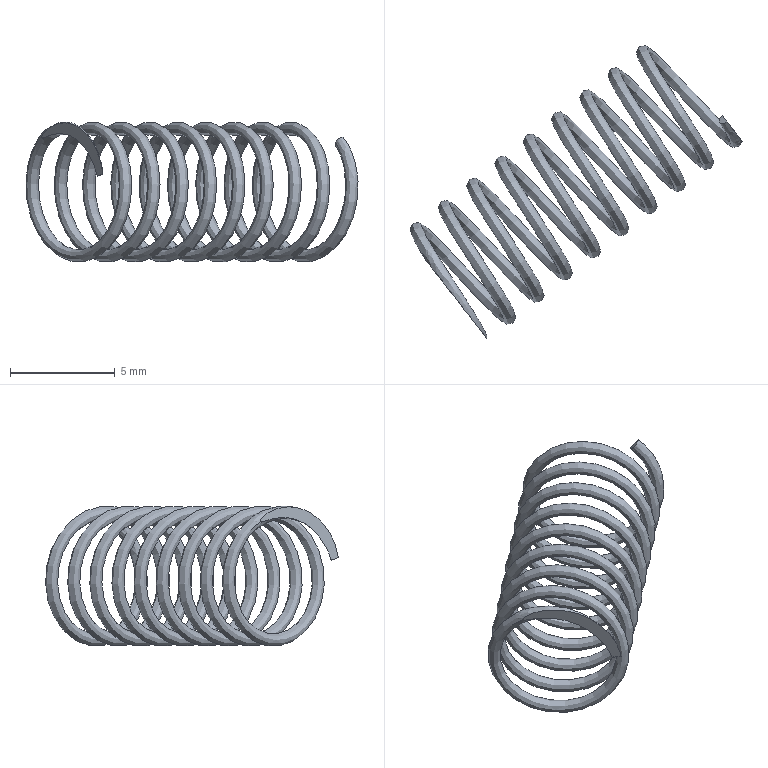Part | NX | features BREP 1 | 1 solid | 5 faces | volume 48.548 mm3 | plane 4 | spline 1
STEP:
#1=CARTESIAN_POINT('',(-3.477,87.158,-116.985));
#2=VERTEX_POINT('',#1);
#3=CARTESIAN_POINT('',(-3.213,86.82,-116.865));
#4=VERTEX_POINT('',#3);
#5=CARTESIAN_POINT('',(-3.345,86.989,-116.925));
#6=DIRECTION('',(0.5927,-0.7586,0.2704));
#7=VECTOR('',#6,1000.);
#8=LINE('',#5,#7);
#9=EDGE_CURVE('',#2,#4,#8,.T.);
#10=ORIENTED_EDGE('',*,*,#9,.F.);
#11=CARTESIAN_POINT('',(-3.213,86.82,-116.865));
#12=CARTESIAN_POINT('',(-3.181,86.983,-116.896));
#13=CARTESIAN_POINT('',(-3.311,87.149,-116.955));
#14=CARTESIAN_POINT('',(-3.477,87.157,-116.985));
#15=B_SPLINE_CURVE_WITH_KNOTS('',3,(#11,#12,#13,#14),.UNSPECIFIED.,.F.,.F.,(4,4),(0.,0.0004991),.UNSPECIFIED.);
#16=EDGE_CURVE('',#4,#2,#15,.T.);
#17=ORIENTED_EDGE('',*,*,#16,.F.);
#18=EDGE_LOOP('',(#10,#17));
#19=FACE_BOUND('',#18,.T.);
#20=CARTESIAN_POINT('',(-3.502,86.866,-116.925));
#21=DIRECTION('',(-0.1665,0.2131,0.9627));
#22=DIRECTION('',(0.788,0.6157,0.));
#23=AXIS2_PLACEMENT_3D('',#20,#21,#22);
#24=PLANE('',#23);
#25=ADVANCED_FACE('',(#19),#24,.F.);
#26=CARTESIAN_POINT('',(8.032,97.44,-115.592));
#27=VERTEX_POINT('',#26);
#28=CARTESIAN_POINT('',(7.91,97.109,-115.357));
#29=VERTEX_POINT('',#28);
#30=CARTESIAN_POINT('',(8.147,97.294,-115.357));
#31=DIRECTION('',(-0.4831,0.6183,0.6199));
#32=DIRECTION('',(-0.788,-0.6157,0.));
#33=AXIS2_PLACEMENT_3D('',#30,#31,#32);
#34=CIRCLE('',#33,0.3);
#35=EDGE_CURVE('',#27,#29,#34,.T.);
#36=ORIENTED_EDGE('',*,*,#35,.F.);
#37=CARTESIAN_POINT('',(8.261,97.147,-115.121));
#38=VERTEX_POINT('',#37);
#39=CARTESIAN_POINT('',(8.032,97.44,-115.592));
#40=CARTESIAN_POINT('',(8.311,97.083,-115.95));
#41=CARTESIAN_POINT('',(8.572,96.75,-116.555));
#42=CARTESIAN_POINT('',(8.721,96.559,-117.384));
#43=CARTESIAN_POINT('',(8.758,96.511,-117.734));
#44=CARTESIAN_POINT('',(8.776,96.489,-118.029));
#45=CARTESIAN_POINT('',(8.787,96.475,-118.188));
#46=CARTESIAN_POINT('',(8.798,96.46,-118.373));
#47=CARTESIAN_POINT('',(8.887,96.346,-118.311));
#48=CARTESIAN_POINT('',(8.925,96.298,-118.048));
#49=CARTESIAN_POINT('',(8.977,96.232,-117.718));
#50=CARTESIAN_POINT('',(8.979,96.228,-117.148));
#51=CARTESIAN_POINT('',(8.889,96.344,-116.453));
#52=CARTESIAN_POINT('',(8.641,96.662,-115.706));
#53=CARTESIAN_POINT('',(8.398,96.972,-115.297));
#54=CARTESIAN_POINT('',(8.261,97.147,-115.121));
#55=B_SPLINE_CURVE_WITH_KNOTS('',3,(#39,#40,#41,#42,#43,#44,#45,#46,#47,#48,#49,#50,#51,#52,#53,#54),.UNSPECIFIED.,.F.,.F.,(4,1,1,1,1,1,1,1,1,1,1,1,1,4),(0.,0.001724,0.002155,0.002586,0.002802,0.003017,0.003125,0.003233,0.003448,0.003879,0.00431,0.005172,0.006034,0.006896),.UNSPECIFIED.);
#56=EDGE_CURVE('',#27,#38,#55,.T.);
#57=ORIENTED_EDGE('',*,*,#56,.T.);
#58=CARTESIAN_POINT('',(8.147,97.294,-115.357));
#59=DIRECTION('',(-0.4831,0.6183,0.6199));
#60=DIRECTION('',(-0.788,-0.6157,0.));
#61=AXIS2_PLACEMENT_3D('',#58,#59,#60);
#62=CIRCLE('',#61,0.3);
#63=EDGE_CURVE('',#29,#38,#62,.T.);
#64=ORIENTED_EDGE('',*,*,#63,.F.);
#65=EDGE_LOOP('',(#36,#57,#64));
#66=FACE_BOUND('',#65,.T.);
#67=CARTESIAN_POINT('',(-3.213,86.82,-116.865));
#68=CARTESIAN_POINT('',(-3.27,86.893,-116.4));
#69=CARTESIAN_POINT('',(-3.527,87.222,-115.533));
#70=CARTESIAN_POINT('',(-4.113,87.971,-114.786));
#71=CARTESIAN_POINT('',(-4.66,88.672,-114.483));
#72=CARTESIAN_POINT('',(-5.095,89.229,-114.412));
#73=CARTESIAN_POINT('',(-5.529,89.784,-114.512));
#74=CARTESIAN_POINT('',(-5.831,90.171,-114.709));
#75=CARTESIAN_POINT('',(-6.016,90.408,-114.909));
#76=CARTESIAN_POINT('',(-6.078,90.487,-115.));
#77=CARTESIAN_POINT('',(-6.139,90.566,-115.105));
#78=CARTESIAN_POINT('',(-6.087,90.498,-115.194));
#79=CARTESIAN_POINT('',(-5.948,90.32,-115.1));
#80=CARTESIAN_POINT('',(-5.779,90.104,-115.048));
#81=CARTESIAN_POINT('',(-5.487,89.73,-114.95));
#82=CARTESIAN_POINT('',(-5.125,89.268,-114.935));
#83=CARTESIAN_POINT('',(-4.254,88.152,-115.192));
#84=CARTESIAN_POINT('',(-3.686,87.426,-116.093));
#85=CARTESIAN_POINT('',(-3.477,87.158,-116.985));
#86=B_SPLINE_CURVE_WITH_KNOTS('',3,(#67,#68,#69,#70,#71,#72,#73,#74,#75,#76,#77,#78,#79,#80,#81,#82,#83,#84,#85),.UNSPECIFIED.,.F.,.F.,(4,1,1,1,1,1,1,1,1,1,1,1,1,1,1,1,4),(0.,0.001414,0.002829,0.003536,0.004243,0.00495,0.005658,0.005834,0.006011,0.0061,0.006188,0.006365,0.006719,0.007072,0.007779,0.008487,0.01132),.UNSPECIFIED.);
#87=EDGE_CURVE('',#4,#2,#86,.T.);
#88=ORIENTED_EDGE('',*,*,#87,.F.);
#89=ORIENTED_EDGE('',*,*,#16,.T.);
#90=EDGE_LOOP('',(#88,#89));
#91=FACE_BOUND('',#90,.T.);
#92=CARTESIAN_POINT('',(7.91,97.109,-115.357));
#93=CARTESIAN_POINT('',(8.648,95.932,-116.448));
#94=CARTESIAN_POINT('',(8.379,96.045,-118.191));
#95=CARTESIAN_POINT('',(8.11,96.158,-119.933));
#96=CARTESIAN_POINT('',(6.99,97.359,-120.584));
#97=CARTESIAN_POINT('',(5.87,98.56,-121.235));
#98=CARTESIAN_POINT('',(4.907,99.561,-120.143));
#99=CARTESIAN_POINT('',(3.944,100.562,-119.052));
#100=CARTESIAN_POINT('',(3.988,100.274,-117.309));
#101=CARTESIAN_POINT('',(4.032,99.985,-115.567));
#102=CARTESIAN_POINT('',(4.927,98.608,-114.916));
#103=CARTESIAN_POINT('',(5.821,97.231,-114.265));
#104=CARTESIAN_POINT('',(6.559,96.054,-115.357));
#105=CARTESIAN_POINT('',(7.298,94.877,-116.448));
#106=CARTESIAN_POINT('',(7.028,94.99,-118.191));
#107=CARTESIAN_POINT('',(6.759,95.102,-119.933));
#108=CARTESIAN_POINT('',(5.639,96.304,-120.584));
#109=CARTESIAN_POINT('',(4.519,97.505,-121.235));
#110=CARTESIAN_POINT('',(3.556,98.506,-120.143));
#111=CARTESIAN_POINT('',(2.593,99.507,-119.052));
#112=CARTESIAN_POINT('',(2.637,99.218,-117.309));
#113=CARTESIAN_POINT('',(2.681,98.93,-115.567));
#114=CARTESIAN_POINT('',(3.576,97.552,-114.916));
#115=CARTESIAN_POINT('',(4.47,96.175,-114.265));
#116=CARTESIAN_POINT('',(5.209,94.998,-115.357));
#117=CARTESIAN_POINT('',(5.947,93.822,-116.448));
#118=CARTESIAN_POINT('',(5.677,93.934,-118.191));
#119=CARTESIAN_POINT('',(5.408,94.047,-119.933));
#120=CARTESIAN_POINT('',(4.288,95.248,-120.584));
#121=CARTESIAN_POINT('',(3.168,96.45,-121.235));
#122=CARTESIAN_POINT('',(2.205,97.45,-120.143));
#123=CARTESIAN_POINT('',(1.242,98.451,-119.052));
#124=CARTESIAN_POINT('',(1.286,98.163,-117.309));
#125=CARTESIAN_POINT('',(1.33,97.874,-115.567));
#126=CARTESIAN_POINT('',(2.225,96.497,-114.916));
#127=CARTESIAN_POINT('',(3.12,95.12,-114.265));
#128=CARTESIAN_POINT('',(3.858,93.943,-115.357));
#129=CARTESIAN_POINT('',(4.596,92.766,-116.448));
#130=CARTESIAN_POINT('',(4.327,92.879,-118.191));
#131=CARTESIAN_POINT('',(4.057,92.991,-119.933));
#132=CARTESIAN_POINT('',(2.937,94.193,-120.584));
#133=CARTESIAN_POINT('',(1.817,95.394,-121.235));
#134=CARTESIAN_POINT('',(0.8542,96.395,-120.143));
#135=CARTESIAN_POINT('',(-0.1091,97.396,-119.052));
#136=CARTESIAN_POINT('',(-0.06498,97.107,-117.309));
#137=CARTESIAN_POINT('',(-0.02088,96.819,-115.567));
#138=CARTESIAN_POINT('',(0.8739,95.442,-114.916));
#139=CARTESIAN_POINT('',(1.769,94.064,-114.265));
#140=CARTESIAN_POINT('',(2.507,92.888,-115.357));
#141=CARTESIAN_POINT('',(3.245,91.711,-116.448));
#142=CARTESIAN_POINT('',(2.976,91.823,-118.191));
#143=CARTESIAN_POINT('',(2.706,91.936,-119.933));
#144=CARTESIAN_POINT('',(1.587,93.137,-120.584));
#145=CARTESIAN_POINT('',(0.4666,94.339,-121.235));
#146=CARTESIAN_POINT('',(-0.4967,95.34,-120.143));
#147=CARTESIAN_POINT('',(-1.46,96.34,-119.052));
#148=CARTESIAN_POINT('',(-1.416,96.052,-117.309));
#149=CARTESIAN_POINT('',(-1.372,95.764,-115.567));
#150=CARTESIAN_POINT('',(-0.477,94.386,-114.916));
#151=CARTESIAN_POINT('',(0.4178,93.009,-114.265));
#152=CARTESIAN_POINT('',(1.156,91.832,-115.357));
#153=CARTESIAN_POINT('',(1.894,90.655,-116.448));
#154=CARTESIAN_POINT('',(1.625,90.768,-118.191));
#155=CARTESIAN_POINT('',(1.356,90.88,-119.933));
#156=CARTESIAN_POINT('',(0.2356,92.082,-120.584));
#157=CARTESIAN_POINT('',(-0.8843,93.283,-121.235));
#158=CARTESIAN_POINT('',(-1.848,94.284,-120.143));
#159=CARTESIAN_POINT('',(-2.811,95.285,-119.052));
#160=CARTESIAN_POINT('',(-2.767,94.997,-117.309));
#161=CARTESIAN_POINT('',(-2.723,94.708,-115.567));
#162=CARTESIAN_POINT('',(-1.828,93.331,-114.916));
#163=CARTESIAN_POINT('',(-0.9331,91.953,-114.265));
#164=CARTESIAN_POINT('',(-0.1949,90.777,-115.357));
#165=CARTESIAN_POINT('',(0.5432,89.6,-116.448));
#166=CARTESIAN_POINT('',(0.2739,89.712,-118.191));
#167=CARTESIAN_POINT('',(0.004697,89.825,-119.933));
#168=CARTESIAN_POINT('',(-1.115,91.026,-120.584));
#169=CARTESIAN_POINT('',(-2.235,92.228,-121.235));
#170=CARTESIAN_POINT('',(-3.198,93.229,-120.143));
#171=CARTESIAN_POINT('',(-4.162,94.23,-119.052));
#172=CARTESIAN_POINT('',(-4.118,93.941,-117.309));
#173=CARTESIAN_POINT('',(-4.074,93.653,-115.567));
#174=CARTESIAN_POINT('',(-3.179,92.275,-114.916));
#175=CARTESIAN_POINT('',(-2.284,90.898,-114.265));
#176=CARTESIAN_POINT('',(-1.546,89.721,-115.357));
#177=CARTESIAN_POINT('',(-0.8077,88.544,-116.448));
#178=CARTESIAN_POINT('',(-1.077,88.657,-118.191));
#179=CARTESIAN_POINT('',(-1.346,88.77,-119.933));
#180=CARTESIAN_POINT('',(-2.466,89.971,-120.584));
#181=CARTESIAN_POINT('',(-3.586,91.172,-121.235));
#182=CARTESIAN_POINT('',(-4.549,92.173,-120.143));
#183=CARTESIAN_POINT('',(-5.513,93.174,-119.052));
#184=CARTESIAN_POINT('',(-5.468,92.886,-117.309));
#185=CARTESIAN_POINT('',(-5.424,92.597,-115.567));
#186=CARTESIAN_POINT('',(-4.53,91.22,-114.916));
#187=CARTESIAN_POINT('',(-3.635,89.843,-114.265));
#188=CARTESIAN_POINT('',(-2.897,88.666,-115.357));
#189=CARTESIAN_POINT('',(-2.159,87.489,-116.448));
#190=CARTESIAN_POINT('',(-2.428,87.602,-118.191));
#191=CARTESIAN_POINT('',(-2.697,87.714,-119.933));
#192=CARTESIAN_POINT('',(-3.817,88.916,-120.584));
#193=CARTESIAN_POINT('',(-4.937,90.117,-121.235));
#194=CARTESIAN_POINT('',(-5.9,91.118,-120.143));
#195=CARTESIAN_POINT('',(-6.863,92.119,-119.052));
#196=CARTESIAN_POINT('',(-6.819,91.83,-117.309));
#197=CARTESIAN_POINT('',(-6.775,91.542,-115.567));
#198=CARTESIAN_POINT('',(-5.88,90.165,-114.916));
#199=CARTESIAN_POINT('',(-4.986,88.787,-114.265));
#200=CARTESIAN_POINT('',(-4.248,87.61,-115.357));
#201=CARTESIAN_POINT('',(-3.832,86.948,-115.971));
#202=CARTESIAN_POINT('',(-3.74,86.68,-116.925));
#203=CARTESIAN_POINT('',(8.139,96.816,-114.886));
#204=CARTESIAN_POINT('',(9.045,95.425,-116.192));
#205=CARTESIAN_POINT('',(8.745,95.577,-118.277));
#206=CARTESIAN_POINT('',(8.445,95.729,-120.363));
#207=CARTESIAN_POINT('',(7.127,97.184,-121.142));
#208=CARTESIAN_POINT('',(5.808,98.639,-121.92));
#209=CARTESIAN_POINT('',(4.678,99.854,-120.614));
#210=CARTESIAN_POINT('',(3.547,101.069,-119.308));
#211=CARTESIAN_POINT('',(3.622,100.742,-117.223));
#212=CARTESIAN_POINT('',(3.697,100.414,-115.137));
#213=CARTESIAN_POINT('',(4.79,98.783,-114.358));
#214=CARTESIAN_POINT('',(5.883,97.152,-113.58));
#215=CARTESIAN_POINT('',(6.788,95.761,-114.886));
#216=CARTESIAN_POINT('',(7.694,94.37,-116.192));
#217=CARTESIAN_POINT('',(7.394,94.522,-118.277));
#218=CARTESIAN_POINT('',(7.094,94.674,-120.363));
#219=CARTESIAN_POINT('',(5.776,96.129,-121.142));
#220=CARTESIAN_POINT('',(4.458,97.584,-121.92));
#221=CARTESIAN_POINT('',(3.327,98.799,-120.614));
#222=CARTESIAN_POINT('',(2.196,100.014,-119.308));
#223=CARTESIAN_POINT('',(2.271,99.686,-117.223));
#224=CARTESIAN_POINT('',(2.346,99.358,-115.137));
#225=CARTESIAN_POINT('',(3.439,97.727,-114.358));
#226=CARTESIAN_POINT('',(4.532,96.096,-113.58));
#227=CARTESIAN_POINT('',(5.438,94.705,-114.886));
#228=CARTESIAN_POINT('',(6.343,93.314,-116.192));
#229=CARTESIAN_POINT('',(6.043,93.466,-118.277));
#230=CARTESIAN_POINT('',(5.743,93.618,-120.363));
#231=CARTESIAN_POINT('',(4.425,95.073,-121.142));
#232=CARTESIAN_POINT('',(3.107,96.528,-121.92));
#233=CARTESIAN_POINT('',(1.976,97.744,-120.614));
#234=CARTESIAN_POINT('',(0.8455,98.959,-119.308));
#235=CARTESIAN_POINT('',(0.9204,98.631,-117.223));
#236=CARTESIAN_POINT('',(0.9953,98.303,-115.137));
#237=CARTESIAN_POINT('',(2.088,96.672,-114.358));
#238=CARTESIAN_POINT('',(3.181,95.041,-113.58));
#239=CARTESIAN_POINT('',(4.087,93.65,-114.886));
#240=CARTESIAN_POINT('',(4.992,92.259,-116.192));
#241=CARTESIAN_POINT('',(4.692,92.411,-118.277));
#242=CARTESIAN_POINT('',(4.392,92.563,-120.363));
#243=CARTESIAN_POINT('',(3.074,94.018,-121.142));
#244=CARTESIAN_POINT('',(1.756,95.473,-121.92));
#245=CARTESIAN_POINT('',(0.6252,96.688,-120.614));
#246=CARTESIAN_POINT('',(-0.5054,97.903,-119.308));
#247=CARTESIAN_POINT('',(-0.4305,97.575,-117.223));
#248=CARTESIAN_POINT('',(-0.3556,97.247,-115.137));
#249=CARTESIAN_POINT('',(0.7374,95.616,-114.358));
#250=CARTESIAN_POINT('',(1.83,93.985,-113.58));
#251=CARTESIAN_POINT('',(2.736,92.594,-114.886));
#252=CARTESIAN_POINT('',(3.641,91.203,-116.192));
#253=CARTESIAN_POINT('',(3.341,91.355,-118.277));
#254=CARTESIAN_POINT('',(3.041,91.507,-120.363));
#255=CARTESIAN_POINT('',(1.723,92.963,-121.142));
#256=CARTESIAN_POINT('',(0.4049,94.418,-121.92));
#257=CARTESIAN_POINT('',(-0.7257,95.633,-120.614));
#258=CARTESIAN_POINT('',(-1.856,96.848,-119.308));
#259=CARTESIAN_POINT('',(-1.781,96.52,-117.223));
#260=CARTESIAN_POINT('',(-1.706,96.192,-115.137));
#261=CARTESIAN_POINT('',(-0.6135,94.561,-114.358));
#262=CARTESIAN_POINT('',(0.4795,92.93,-113.58));
#263=CARTESIAN_POINT('',(1.385,91.539,-114.886));
#264=CARTESIAN_POINT('',(2.29,90.148,-116.192));
#265=CARTESIAN_POINT('',(1.99,90.3,-118.277));
#266=CARTESIAN_POINT('',(1.69,90.452,-120.363));
#267=CARTESIAN_POINT('',(0.3722,91.907,-121.142));
#268=CARTESIAN_POINT('',(-0.9459,93.362,-121.92));
#269=CARTESIAN_POINT('',(-2.077,94.577,-120.614));
#270=CARTESIAN_POINT('',(-3.207,95.792,-119.308));
#271=CARTESIAN_POINT('',(-3.132,95.464,-117.223));
#272=CARTESIAN_POINT('',(-3.057,95.136,-115.137));
#273=CARTESIAN_POINT('',(-1.964,93.506,-114.358));
#274=CARTESIAN_POINT('',(-0.8714,91.875,-113.58));
#275=CARTESIAN_POINT('',(0.03406,90.484,-114.886));
#276=CARTESIAN_POINT('',(0.9395,89.093,-116.192));
#277=CARTESIAN_POINT('',(0.6395,89.245,-118.277));
#278=CARTESIAN_POINT('',(0.3394,89.397,-120.363));
#279=CARTESIAN_POINT('',(-0.9787,90.852,-121.142));
#280=CARTESIAN_POINT('',(-2.297,92.307,-121.92));
#281=CARTESIAN_POINT('',(-3.427,93.522,-120.614));
#282=CARTESIAN_POINT('',(-4.558,94.737,-119.308));
#283=CARTESIAN_POINT('',(-4.483,94.409,-117.223));
#284=CARTESIAN_POINT('',(-4.408,94.081,-115.137));
#285=CARTESIAN_POINT('',(-3.315,92.45,-114.358));
#286=CARTESIAN_POINT('',(-2.222,90.819,-113.58));
#287=CARTESIAN_POINT('',(-1.317,89.428,-114.886));
#288=CARTESIAN_POINT('',(-0.4113,88.037,-116.192));
#289=CARTESIAN_POINT('',(-0.7114,88.189,-118.277));
#290=CARTESIAN_POINT('',(-1.011,88.341,-120.363));
#291=CARTESIAN_POINT('',(-2.33,89.796,-121.142));
#292=CARTESIAN_POINT('',(-3.648,91.251,-121.92));
#293=CARTESIAN_POINT('',(-4.778,92.466,-120.614));
#294=CARTESIAN_POINT('',(-5.909,93.682,-119.308));
#295=CARTESIAN_POINT('',(-5.834,93.354,-117.223));
#296=CARTESIAN_POINT('',(-5.759,93.026,-115.137));
#297=CARTESIAN_POINT('',(-4.666,91.395,-114.358));
#298=CARTESIAN_POINT('',(-3.573,89.764,-113.58));
#299=CARTESIAN_POINT('',(-2.668,88.373,-114.886));
#300=CARTESIAN_POINT('',(-1.762,86.982,-116.192));
#301=CARTESIAN_POINT('',(-2.062,87.134,-118.277));
#302=CARTESIAN_POINT('',(-2.362,87.286,-120.363));
#303=CARTESIAN_POINT('',(-3.68,88.741,-121.142));
#304=CARTESIAN_POINT('',(-4.999,90.196,-121.92));
#305=CARTESIAN_POINT('',(-6.129,91.411,-120.614));
#306=CARTESIAN_POINT('',(-7.26,92.626,-119.308));
#307=CARTESIAN_POINT('',(-7.185,92.298,-117.223));
#308=CARTESIAN_POINT('',(-7.11,91.97,-115.137));
#309=CARTESIAN_POINT('',(-6.017,90.339,-114.358));
#310=CARTESIAN_POINT('',(-4.924,88.708,-113.58));
#311=CARTESIAN_POINT('',(-4.019,87.317,-114.886));
#312=CARTESIAN_POINT('',(-3.509,86.534,-115.621));
#313=CARTESIAN_POINT('',(-3.384,86.225,-116.763));
#314=CARTESIAN_POINT('',(8.612,97.185,-114.886));
#315=CARTESIAN_POINT('',(9.518,95.795,-116.192));
#316=CARTESIAN_POINT('',(9.218,95.947,-118.277));
#317=CARTESIAN_POINT('',(8.917,96.099,-120.363));
#318=CARTESIAN_POINT('',(7.599,97.554,-121.142));
#319=CARTESIAN_POINT('',(6.281,99.009,-121.92));
#320=CARTESIAN_POINT('',(5.151,100.224,-120.614));
#321=CARTESIAN_POINT('',(4.02,101.439,-119.308));
#322=CARTESIAN_POINT('',(4.095,101.111,-117.223));
#323=CARTESIAN_POINT('',(4.17,100.783,-115.137));
#324=CARTESIAN_POINT('',(5.263,99.152,-114.358));
#325=CARTESIAN_POINT('',(6.356,97.521,-113.58));
#326=CARTESIAN_POINT('',(7.261,96.13,-114.886));
#327=CARTESIAN_POINT('',(8.167,94.739,-116.192));
#328=CARTESIAN_POINT('',(7.867,94.891,-118.277));
#329=CARTESIAN_POINT('',(7.567,95.043,-120.363));
#330=CARTESIAN_POINT('',(6.248,96.498,-121.142));
#331=CARTESIAN_POINT('',(4.93,97.953,-121.92));
#332=CARTESIAN_POINT('',(3.8,99.168,-120.614));
#333=CARTESIAN_POINT('',(2.669,100.383,-119.308));
#334=CARTESIAN_POINT('',(2.744,100.055,-117.223));
#335=CARTESIAN_POINT('',(2.819,99.728,-115.137));
#336=CARTESIAN_POINT('',(3.912,98.097,-114.358));
#337=CARTESIAN_POINT('',(5.005,96.466,-113.58));
#338=CARTESIAN_POINT('',(5.91,95.075,-114.886));
#339=CARTESIAN_POINT('',(6.816,93.684,-116.192));
#340=CARTESIAN_POINT('',(6.516,93.836,-118.277));
#341=CARTESIAN_POINT('',(6.216,93.988,-120.363));
#342=CARTESIAN_POINT('',(4.898,95.443,-121.142));
#343=CARTESIAN_POINT('',(3.579,96.898,-121.92));
#344=CARTESIAN_POINT('',(2.449,98.113,-120.614));
#345=CARTESIAN_POINT('',(1.318,99.328,-119.308));
#346=CARTESIAN_POINT('',(1.393,99.,-117.223));
#347=CARTESIAN_POINT('',(1.468,98.672,-115.137));
#348=CARTESIAN_POINT('',(2.561,97.041,-114.358));
#349=CARTESIAN_POINT('',(3.654,95.41,-113.58));
#350=CARTESIAN_POINT('',(4.559,94.019,-114.886));
#351=CARTESIAN_POINT('',(5.465,92.628,-116.192));
#352=CARTESIAN_POINT('',(5.165,92.78,-118.277));
#353=CARTESIAN_POINT('',(4.865,92.932,-120.363));
#354=CARTESIAN_POINT('',(3.547,94.387,-121.142));
#355=CARTESIAN_POINT('',(2.229,95.842,-121.92));
#356=CARTESIAN_POINT('',(1.098,97.058,-120.614));
#357=CARTESIAN_POINT('',(-0.03261,98.273,-119.308));
#358=CARTESIAN_POINT('',(0.04231,97.945,-117.223));
#359=CARTESIAN_POINT('',(0.1172,97.617,-115.137));
#360=CARTESIAN_POINT('',(1.21,95.986,-114.358));
#361=CARTESIAN_POINT('',(2.303,94.355,-113.58));
#362=CARTESIAN_POINT('',(3.209,92.964,-114.886));
#363=CARTESIAN_POINT('',(4.114,91.573,-116.192));
#364=CARTESIAN_POINT('',(3.814,91.725,-118.277));
#365=CARTESIAN_POINT('',(3.514,91.877,-120.363));
#366=CARTESIAN_POINT('',(2.196,93.332,-121.142));
#367=CARTESIAN_POINT('',(0.8777,94.787,-121.92));
#368=CARTESIAN_POINT('',(-0.2529,96.002,-120.614));
#369=CARTESIAN_POINT('',(-1.383,97.217,-119.308));
#370=CARTESIAN_POINT('',(-1.309,96.889,-117.223));
#371=CARTESIAN_POINT('',(-1.234,96.561,-115.137));
#372=CARTESIAN_POINT('',(-0.1407,94.93,-114.358));
#373=CARTESIAN_POINT('',(0.9523,93.299,-113.58));
#374=CARTESIAN_POINT('',(1.858,91.908,-114.886));
#375=CARTESIAN_POINT('',(2.763,90.517,-116.192));
#376=CARTESIAN_POINT('',(2.463,90.669,-118.277));
#377=CARTESIAN_POINT('',(2.163,90.821,-120.363));
#378=CARTESIAN_POINT('',(0.845,92.277,-121.142));
#379=CARTESIAN_POINT('',(-0.4731,93.732,-121.92));
#380=CARTESIAN_POINT('',(-1.604,94.947,-120.614));
#381=CARTESIAN_POINT('',(-2.734,96.162,-119.308));
#382=CARTESIAN_POINT('',(-2.659,95.834,-117.223));
#383=CARTESIAN_POINT('',(-2.585,95.506,-115.137));
#384=CARTESIAN_POINT('',(-1.492,93.875,-114.358));
#385=CARTESIAN_POINT('',(-0.3986,92.244,-113.58));
#386=CARTESIAN_POINT('',(0.5069,90.853,-114.886));
#387=CARTESIAN_POINT('',(1.412,89.462,-116.192));
#388=CARTESIAN_POINT('',(1.112,89.614,-118.277));
#389=CARTESIAN_POINT('',(0.8122,89.766,-120.363));
#390=CARTESIAN_POINT('',(-0.5059,91.221,-121.142));
#391=CARTESIAN_POINT('',(-1.824,92.676,-121.92));
#392=CARTESIAN_POINT('',(-2.955,93.891,-120.614));
#393=CARTESIAN_POINT('',(-4.085,95.106,-119.308));
#394=CARTESIAN_POINT('',(-4.01,94.778,-117.223));
#395=CARTESIAN_POINT('',(-3.935,94.45,-115.137));
#396=CARTESIAN_POINT('',(-2.842,92.82,-114.358));
#397=CARTESIAN_POINT('',(-1.749,91.189,-113.58));
#398=CARTESIAN_POINT('',(-0.844,89.798,-114.886));
#399=CARTESIAN_POINT('',(0.06146,88.407,-116.192));
#400=CARTESIAN_POINT('',(-0.2386,88.559,-118.277));
#401=CARTESIAN_POINT('',(-0.5387,88.711,-120.363));
#402=CARTESIAN_POINT('',(-1.857,90.166,-121.142));
#403=CARTESIAN_POINT('',(-3.175,91.621,-121.92));
#404=CARTESIAN_POINT('',(-4.306,92.836,-120.614));
#405=CARTESIAN_POINT('',(-5.436,94.051,-119.308));
#406=CARTESIAN_POINT('',(-5.361,93.723,-117.223));
#407=CARTESIAN_POINT('',(-5.286,93.395,-115.137));
#408=CARTESIAN_POINT('',(-4.193,91.764,-114.358));
#409=CARTESIAN_POINT('',(-3.1,90.133,-113.58));
#410=CARTESIAN_POINT('',(-2.195,88.742,-114.886));
#411=CARTESIAN_POINT('',(-1.289,87.351,-116.192));
#412=CARTESIAN_POINT('',(-1.589,87.503,-118.277));
#413=CARTESIAN_POINT('',(-1.89,87.655,-120.363));
#414=CARTESIAN_POINT('',(-3.208,89.11,-121.142));
#415=CARTESIAN_POINT('',(-4.526,90.565,-121.92));
#416=CARTESIAN_POINT('',(-5.656,91.78,-120.614));
#417=CARTESIAN_POINT('',(-6.787,92.995,-119.308));
#418=CARTESIAN_POINT('',(-6.712,92.668,-117.223));
#419=CARTESIAN_POINT('',(-6.637,92.34,-115.137));
#420=CARTESIAN_POINT('',(-5.544,90.709,-114.358));
#421=CARTESIAN_POINT('',(-4.451,89.078,-113.58));
#422=CARTESIAN_POINT('',(-3.546,87.687,-114.886));
#423=CARTESIAN_POINT('',(-3.036,86.904,-115.621));
#424=CARTESIAN_POINT('',(-2.911,86.594,-116.763));
#425=CARTESIAN_POINT('',(8.383,97.479,-115.357));
#426=CARTESIAN_POINT('',(9.121,96.302,-116.448));
#427=CARTESIAN_POINT('',(8.852,96.414,-118.191));
#428=CARTESIAN_POINT('',(8.583,96.527,-119.933));
#429=CARTESIAN_POINT('',(7.463,97.728,-120.584));
#430=CARTESIAN_POINT('',(6.343,98.93,-121.235));
#431=CARTESIAN_POINT('',(5.38,99.931,-120.143));
#432=CARTESIAN_POINT('',(4.416,100.932,-119.052));
#433=CARTESIAN_POINT('',(4.46,100.643,-117.309));
#434=CARTESIAN_POINT('',(4.505,100.355,-115.567));
#435=CARTESIAN_POINT('',(5.399,98.977,-114.916));
#436=CARTESIAN_POINT('',(6.294,97.6,-114.265));
#437=CARTESIAN_POINT('',(7.032,96.423,-115.357));
#438=CARTESIAN_POINT('',(7.77,95.246,-116.448));
#439=CARTESIAN_POINT('',(7.501,95.359,-118.191));
#440=CARTESIAN_POINT('',(7.232,95.472,-119.933));
#441=CARTESIAN_POINT('',(6.112,96.673,-120.584));
#442=CARTESIAN_POINT('',(4.992,97.874,-121.235));
#443=CARTESIAN_POINT('',(4.029,98.875,-120.143));
#444=CARTESIAN_POINT('',(3.065,99.876,-119.052));
#445=CARTESIAN_POINT('',(3.11,99.588,-117.309));
#446=CARTESIAN_POINT('',(3.154,99.299,-115.567));
#447=CARTESIAN_POINT('',(4.048,97.922,-114.916));
#448=CARTESIAN_POINT('',(4.943,96.545,-114.265));
#449=CARTESIAN_POINT('',(5.681,95.368,-115.357));
#450=CARTESIAN_POINT('',(6.419,94.191,-116.448));
#451=CARTESIAN_POINT('',(6.15,94.304,-118.191));
#452=CARTESIAN_POINT('',(5.881,94.416,-119.933));
#453=CARTESIAN_POINT('',(4.761,95.618,-120.584));
#454=CARTESIAN_POINT('',(3.641,96.819,-121.235));
#455=CARTESIAN_POINT('',(2.678,97.82,-120.143));
#456=CARTESIAN_POINT('',(1.715,98.821,-119.052));
#457=CARTESIAN_POINT('',(1.759,98.532,-117.309));
#458=CARTESIAN_POINT('',(1.803,98.244,-115.567));
#459=CARTESIAN_POINT('',(2.698,96.866,-114.916));
#460=CARTESIAN_POINT('',(3.592,95.489,-114.265));
#461=CARTESIAN_POINT('',(4.331,94.312,-115.357));
#462=CARTESIAN_POINT('',(5.069,93.136,-116.448));
#463=CARTESIAN_POINT('',(4.799,93.248,-118.191));
#464=CARTESIAN_POINT('',(4.53,93.361,-119.933));
#465=CARTESIAN_POINT('',(3.41,94.562,-120.584));
#466=CARTESIAN_POINT('',(2.29,95.764,-121.235));
#467=CARTESIAN_POINT('',(1.327,96.764,-120.143));
#468=CARTESIAN_POINT('',(0.3637,97.765,-119.052));
#469=CARTESIAN_POINT('',(0.4078,97.477,-117.309));
#470=CARTESIAN_POINT('',(0.4519,97.188,-115.567));
#471=CARTESIAN_POINT('',(1.347,95.811,-114.916));
#472=CARTESIAN_POINT('',(2.242,94.434,-114.265));
#473=CARTESIAN_POINT('',(2.98,93.257,-115.357));
#474=CARTESIAN_POINT('',(3.718,92.08,-116.448));
#475=CARTESIAN_POINT('',(3.448,92.193,-118.191));
#476=CARTESIAN_POINT('',(3.179,92.305,-119.933));
#477=CARTESIAN_POINT('',(2.059,93.507,-120.584));
#478=CARTESIAN_POINT('',(0.9394,94.708,-121.235));
#479=CARTESIAN_POINT('',(-0.02388,95.709,-120.143));
#480=CARTESIAN_POINT('',(-0.9871,96.71,-119.052));
#481=CARTESIAN_POINT('',(-0.9431,96.421,-117.309));
#482=CARTESIAN_POINT('',(-0.899,96.133,-115.567));
#483=CARTESIAN_POINT('',(-0.00416,94.756,-114.916));
#484=CARTESIAN_POINT('',(0.8906,93.378,-114.265));
#485=CARTESIAN_POINT('',(1.629,92.201,-115.357));
#486=CARTESIAN_POINT('',(2.367,91.025,-116.448));
#487=CARTESIAN_POINT('',(2.098,91.137,-118.191));
#488=CARTESIAN_POINT('',(1.828,91.25,-119.933));
#489=CARTESIAN_POINT('',(0.7084,92.451,-120.584));
#490=CARTESIAN_POINT('',(-0.4115,93.653,-121.235));
#491=CARTESIAN_POINT('',(-1.375,94.654,-120.143));
#492=CARTESIAN_POINT('',(-2.338,95.654,-119.052));
#493=CARTESIAN_POINT('',(-2.294,95.366,-117.309));
#494=CARTESIAN_POINT('',(-2.25,95.077,-115.567));
#495=CARTESIAN_POINT('',(-1.355,93.7,-114.916));
#496=CARTESIAN_POINT('',(-0.4602,92.323,-114.265));
#497=CARTESIAN_POINT('',(0.2779,91.146,-115.357));
#498=CARTESIAN_POINT('',(1.016,89.969,-116.448));
#499=CARTESIAN_POINT('',(0.7467,90.082,-118.191));
#500=CARTESIAN_POINT('',(0.4775,90.194,-119.933));
#501=CARTESIAN_POINT('',(-0.6424,91.396,-120.584));
#502=CARTESIAN_POINT('',(-1.762,92.597,-121.235));
#503=CARTESIAN_POINT('',(-2.726,93.598,-120.143));
#504=CARTESIAN_POINT('',(-3.689,94.599,-119.052));
#505=CARTESIAN_POINT('',(-3.645,94.311,-117.309));
#506=CARTESIAN_POINT('',(-3.601,94.022,-115.567));
#507=CARTESIAN_POINT('',(-2.706,92.645,-114.916));
#508=CARTESIAN_POINT('',(-1.811,91.267,-114.265));
#509=CARTESIAN_POINT('',(-1.073,90.091,-115.357));
#510=CARTESIAN_POINT('',(-0.3349,88.914,-116.448));
#511=CARTESIAN_POINT('',(-0.6041,89.026,-118.191));
#512=CARTESIAN_POINT('',(-0.8734,89.139,-119.933));
#513=CARTESIAN_POINT('',(-1.993,90.34,-120.584));
#514=CARTESIAN_POINT('',(-3.113,91.542,-121.235));
#515=CARTESIAN_POINT('',(-4.077,92.543,-120.143));
#516=CARTESIAN_POINT('',(-5.04,93.544,-119.052));
#517=CARTESIAN_POINT('',(-4.996,93.255,-117.309));
#518=CARTESIAN_POINT('',(-4.952,92.967,-115.567));
#519=CARTESIAN_POINT('',(-4.057,91.589,-114.916));
#520=CARTESIAN_POINT('',(-3.162,90.212,-114.265));
#521=CARTESIAN_POINT('',(-2.424,89.035,-115.357));
#522=CARTESIAN_POINT('',(-1.686,87.858,-116.448));
#523=CARTESIAN_POINT('',(-1.955,87.971,-118.191));
#524=CARTESIAN_POINT('',(-2.224,88.084,-119.933));
#525=CARTESIAN_POINT('',(-3.344,89.285,-120.584));
#526=CARTESIAN_POINT('',(-4.464,90.486,-121.235));
#527=CARTESIAN_POINT('',(-5.427,91.487,-120.143));
#528=CARTESIAN_POINT('',(-6.391,92.488,-119.052));
#529=CARTESIAN_POINT('',(-6.347,92.2,-117.309));
#530=CARTESIAN_POINT('',(-6.302,91.911,-115.567));
#531=CARTESIAN_POINT('',(-5.408,90.534,-114.916));
#532=CARTESIAN_POINT('',(-4.513,89.157,-114.265));
#533=CARTESIAN_POINT('',(-3.775,87.98,-115.357));
#534=CARTESIAN_POINT('',(-3.359,87.318,-115.971));
#535=CARTESIAN_POINT('',(-3.267,87.049,-116.925));
#536=CARTESIAN_POINT('',(8.154,97.772,-115.828));
#537=CARTESIAN_POINT('',(8.725,96.809,-116.704));
#538=CARTESIAN_POINT('',(8.486,96.882,-118.104));
#539=CARTESIAN_POINT('',(8.248,96.955,-119.504));
#540=CARTESIAN_POINT('',(7.326,97.903,-120.027));
#541=CARTESIAN_POINT('',(6.405,98.851,-120.549));
#542=CARTESIAN_POINT('',(5.609,99.638,-119.672));
#543=CARTESIAN_POINT('',(4.813,100.424,-118.796));
#544=CARTESIAN_POINT('',(4.826,100.175,-117.396));
#545=CARTESIAN_POINT('',(4.839,99.926,-115.996));
#546=CARTESIAN_POINT('',(5.536,98.803,-115.473));
#547=CARTESIAN_POINT('',(6.232,97.679,-114.951));
#548=CARTESIAN_POINT('',(6.803,96.716,-115.828));
#549=CARTESIAN_POINT('',(7.374,95.754,-116.704));
#550=CARTESIAN_POINT('',(7.136,95.827,-118.104));
#551=CARTESIAN_POINT('',(6.897,95.9,-119.504));
#552=CARTESIAN_POINT('',(5.975,96.848,-120.027));
#553=CARTESIAN_POINT('',(5.054,97.795,-120.549));
#554=CARTESIAN_POINT('',(4.258,98.582,-119.672));
#555=CARTESIAN_POINT('',(3.462,99.369,-118.796));
#556=CARTESIAN_POINT('',(3.475,99.12,-117.396));
#557=CARTESIAN_POINT('',(3.488,98.871,-115.996));
#558=CARTESIAN_POINT('',(4.185,97.747,-115.473));
#559=CARTESIAN_POINT('',(4.882,96.623,-114.951));
#560=CARTESIAN_POINT('',(5.452,95.661,-115.828));
#561=CARTESIAN_POINT('',(6.023,94.698,-116.704));
#562=CARTESIAN_POINT('',(5.785,94.771,-118.104));
#563=CARTESIAN_POINT('',(5.546,94.845,-119.504));
#564=CARTESIAN_POINT('',(4.625,95.792,-120.027));
#565=CARTESIAN_POINT('',(3.703,96.74,-120.549));
#566=CARTESIAN_POINT('',(2.907,97.527,-119.672));
#567=CARTESIAN_POINT('',(2.111,98.313,-118.796));
#568=CARTESIAN_POINT('',(2.124,98.064,-117.396));
#569=CARTESIAN_POINT('',(2.137,97.815,-115.996));
#570=CARTESIAN_POINT('',(2.834,96.692,-115.473));
#571=CARTESIAN_POINT('',(3.531,95.568,-114.951));
#572=CARTESIAN_POINT('',(4.102,94.605,-115.828));
#573=CARTESIAN_POINT('',(4.672,93.643,-116.704));
#574=CARTESIAN_POINT('',(4.434,93.716,-118.104));
#575=CARTESIAN_POINT('',(4.195,93.789,-119.504));
#576=CARTESIAN_POINT('',(3.274,94.737,-120.027));
#577=CARTESIAN_POINT('',(2.352,95.685,-120.549));
#578=CARTESIAN_POINT('',(1.556,96.471,-119.672));
#579=CARTESIAN_POINT('',(0.7601,97.258,-118.796));
#580=CARTESIAN_POINT('',(0.7733,97.009,-117.396));
#581=CARTESIAN_POINT('',(0.7866,96.76,-115.996));
#582=CARTESIAN_POINT('',(1.483,95.636,-115.473));
#583=CARTESIAN_POINT('',(2.18,94.513,-114.951));
#584=CARTESIAN_POINT('',(2.751,93.55,-115.828));
#585=CARTESIAN_POINT('',(3.321,92.587,-116.704));
#586=CARTESIAN_POINT('',(3.083,92.661,-118.104));
#587=CARTESIAN_POINT('',(2.845,92.734,-119.504));
#588=CARTESIAN_POINT('',(1.923,93.681,-120.027));
#589=CARTESIAN_POINT('',(1.001,94.629,-120.549));
#590=CARTESIAN_POINT('',(0.2051,95.416,-119.672));
#591=CARTESIAN_POINT('',(-0.5908,96.203,-118.796));
#592=CARTESIAN_POINT('',(-0.5775,95.954,-117.396));
#593=CARTESIAN_POINT('',(-0.5643,95.705,-115.996));
#594=CARTESIAN_POINT('',(0.1324,94.581,-115.473));
#595=CARTESIAN_POINT('',(0.829,93.457,-114.951));
#596=CARTESIAN_POINT('',(1.4,92.495,-115.828));
#597=CARTESIAN_POINT('',(1.971,91.532,-116.704));
#598=CARTESIAN_POINT('',(1.732,91.605,-118.104));
#599=CARTESIAN_POINT('',(1.494,91.678,-119.504));
#600=CARTESIAN_POINT('',(0.5719,92.626,-120.027));
#601=CARTESIAN_POINT('',(-0.3499,93.574,-120.549));
#602=CARTESIAN_POINT('',(-1.146,94.36,-119.672));
#603=CARTESIAN_POINT('',(-1.942,95.147,-118.796));
#604=CARTESIAN_POINT('',(-1.928,94.898,-117.396));
#605=CARTESIAN_POINT('',(-1.915,94.649,-115.996));
#606=CARTESIAN_POINT('',(-1.219,93.525,-115.473));
#607=CARTESIAN_POINT('',(-0.5219,92.402,-114.951));
#608=CARTESIAN_POINT('',(0.04888,91.439,-115.828));
#609=CARTESIAN_POINT('',(0.6197,90.477,-116.704));
#610=CARTESIAN_POINT('',(0.3812,90.55,-118.104));
#611=CARTESIAN_POINT('',(0.1428,90.623,-119.504));
#612=CARTESIAN_POINT('',(-0.779,91.571,-120.027));
#613=CARTESIAN_POINT('',(-1.701,92.518,-120.549));
#614=CARTESIAN_POINT('',(-2.497,93.305,-119.672));
#615=CARTESIAN_POINT('',(-3.293,94.092,-118.796));
#616=CARTESIAN_POINT('',(-3.279,93.843,-117.396));
#617=CARTESIAN_POINT('',(-3.266,93.594,-115.996));
#618=CARTESIAN_POINT('',(-2.569,92.47,-115.473));
#619=CARTESIAN_POINT('',(-1.873,91.346,-114.951));
#620=CARTESIAN_POINT('',(-1.302,90.384,-115.828));
#621=CARTESIAN_POINT('',(-0.7312,89.421,-116.704));
#622=CARTESIAN_POINT('',(-0.9696,89.494,-118.104));
#623=CARTESIAN_POINT('',(-1.208,89.567,-119.504));
#624=CARTESIAN_POINT('',(-2.13,90.515,-120.027));
#625=CARTESIAN_POINT('',(-3.052,91.463,-120.549));
#626=CARTESIAN_POINT('',(-3.848,92.25,-119.672));
#627=CARTESIAN_POINT('',(-4.643,93.036,-118.796));
#628=CARTESIAN_POINT('',(-4.63,92.787,-117.396));
#629=CARTESIAN_POINT('',(-4.617,92.538,-115.996));
#630=CARTESIAN_POINT('',(-3.92,91.415,-115.473));
#631=CARTESIAN_POINT('',(-3.224,90.291,-114.951));
#632=CARTESIAN_POINT('',(-2.653,89.328,-115.828));
#633=CARTESIAN_POINT('',(-2.082,88.366,-116.704));
#634=CARTESIAN_POINT('',(-2.321,88.439,-118.104));
#635=CARTESIAN_POINT('',(-2.559,88.512,-119.504));
#636=CARTESIAN_POINT('',(-3.481,89.46,-120.027));
#637=CARTESIAN_POINT('',(-4.402,90.408,-120.549));
#638=CARTESIAN_POINT('',(-5.198,91.194,-119.672));
#639=CARTESIAN_POINT('',(-5.994,91.981,-118.796));
#640=CARTESIAN_POINT('',(-5.981,91.732,-117.396));
#641=CARTESIAN_POINT('',(-5.968,91.483,-115.996));
#642=CARTESIAN_POINT('',(-5.271,90.359,-115.473));
#643=CARTESIAN_POINT('',(-4.575,89.235,-114.951));
#644=CARTESIAN_POINT('',(-4.004,88.273,-115.828));
#645=CARTESIAN_POINT('',(-3.683,87.731,-116.321));
#646=CARTESIAN_POINT('',(-3.623,87.505,-117.087));
#647=CARTESIAN_POINT('',(7.681,97.402,-115.828));
#648=CARTESIAN_POINT('',(8.252,96.44,-116.704));
#649=CARTESIAN_POINT('',(8.014,96.513,-118.104));
#650=CARTESIAN_POINT('',(7.775,96.586,-119.504));
#651=CARTESIAN_POINT('',(6.853,97.534,-120.027));
#652=CARTESIAN_POINT('',(5.932,98.481,-120.549));
#653=CARTESIAN_POINT('',(5.136,99.268,-119.672));
#654=CARTESIAN_POINT('',(4.34,100.055,-118.796));
#655=CARTESIAN_POINT('',(4.353,99.806,-117.396));
#656=CARTESIAN_POINT('',(4.366,99.557,-115.996));
#657=CARTESIAN_POINT('',(5.063,98.433,-115.473));
#658=CARTESIAN_POINT('',(5.76,97.309,-114.951));
#659=CARTESIAN_POINT('',(6.33,96.347,-115.828));
#660=CARTESIAN_POINT('',(6.901,95.384,-116.704));
#661=CARTESIAN_POINT('',(6.663,95.457,-118.104));
#662=CARTESIAN_POINT('',(6.424,95.531,-119.504));
#663=CARTESIAN_POINT('',(5.503,96.478,-120.027));
#664=CARTESIAN_POINT('',(4.581,97.426,-120.549));
#665=CARTESIAN_POINT('',(3.785,98.213,-119.672));
#666=CARTESIAN_POINT('',(2.989,98.999,-118.796));
#667=CARTESIAN_POINT('',(3.002,98.75,-117.396));
#668=CARTESIAN_POINT('',(3.016,98.501,-115.996));
#669=CARTESIAN_POINT('',(3.712,97.378,-115.473));
#670=CARTESIAN_POINT('',(4.409,96.254,-114.951));
#671=CARTESIAN_POINT('',(4.98,95.291,-115.828));
#672=CARTESIAN_POINT('',(5.55,94.329,-116.704));
#673=CARTESIAN_POINT('',(5.312,94.402,-118.104));
#674=CARTESIAN_POINT('',(5.074,94.475,-119.504));
#675=CARTESIAN_POINT('',(4.152,95.423,-120.027));
#676=CARTESIAN_POINT('',(3.23,96.371,-120.549));
#677=CARTESIAN_POINT('',(2.434,97.157,-119.672));
#678=CARTESIAN_POINT('',(1.638,97.944,-118.796));
#679=CARTESIAN_POINT('',(1.651,97.695,-117.396));
#680=CARTESIAN_POINT('',(1.665,97.446,-115.996));
#681=CARTESIAN_POINT('',(2.361,96.322,-115.473));
#682=CARTESIAN_POINT('',(3.058,95.199,-114.951));
#683=CARTESIAN_POINT('',(3.629,94.236,-115.828));
#684=CARTESIAN_POINT('',(4.199,93.273,-116.704));
#685=CARTESIAN_POINT('',(3.961,93.347,-118.104));
#686=CARTESIAN_POINT('',(3.723,93.42,-119.504));
#687=CARTESIAN_POINT('',(2.801,94.367,-120.027));
#688=CARTESIAN_POINT('',(1.879,95.315,-120.549));
#689=CARTESIAN_POINT('',(1.083,96.102,-119.672));
#690=CARTESIAN_POINT('',(0.2873,96.889,-118.796));
#691=CARTESIAN_POINT('',(0.3005,96.64,-117.396));
#692=CARTESIAN_POINT('',(0.3138,96.391,-115.996));
#693=CARTESIAN_POINT('',(1.01,95.267,-115.473));
#694=CARTESIAN_POINT('',(1.707,94.143,-114.951));
#695=CARTESIAN_POINT('',(2.278,93.181,-115.828));
#696=CARTESIAN_POINT('',(2.849,92.218,-116.704));
#697=CARTESIAN_POINT('',(2.61,92.291,-118.104));
#698=CARTESIAN_POINT('',(2.372,92.364,-119.504));
#699=CARTESIAN_POINT('',(1.45,93.312,-120.027));
#700=CARTESIAN_POINT('',(0.5282,94.26,-120.549));
#701=CARTESIAN_POINT('',(-0.2677,95.046,-119.672));
#702=CARTESIAN_POINT('',(-1.064,95.833,-118.796));
#703=CARTESIAN_POINT('',(-1.05,95.584,-117.396));
#704=CARTESIAN_POINT('',(-1.037,95.335,-115.996));
#705=CARTESIAN_POINT('',(-0.3404,94.211,-115.473));
#706=CARTESIAN_POINT('',(0.3562,93.088,-114.951));
#707=CARTESIAN_POINT('',(0.927,92.125,-115.828));
#708=CARTESIAN_POINT('',(1.498,91.163,-116.704));
#709=CARTESIAN_POINT('',(1.259,91.236,-118.104));
#710=CARTESIAN_POINT('',(1.021,91.309,-119.504));
#711=CARTESIAN_POINT('',(0.09911,92.257,-120.027));
#712=CARTESIAN_POINT('',(-0.8227,93.204,-120.549));
#713=CARTESIAN_POINT('',(-1.619,93.991,-119.672));
#714=CARTESIAN_POINT('',(-2.414,94.778,-118.796));
#715=CARTESIAN_POINT('',(-2.401,94.529,-117.396));
#716=CARTESIAN_POINT('',(-2.388,94.28,-115.996));
#717=CARTESIAN_POINT('',(-1.691,93.156,-115.473));
#718=CARTESIAN_POINT('',(-0.9947,92.032,-114.951));
#719=CARTESIAN_POINT('',(-0.4239,91.07,-115.828));
#720=CARTESIAN_POINT('',(0.1468,90.107,-116.704));
#721=CARTESIAN_POINT('',(-0.09158,90.18,-118.104));
#722=CARTESIAN_POINT('',(-0.33,90.253,-119.504));
#723=CARTESIAN_POINT('',(-1.252,91.201,-120.027));
#724=CARTESIAN_POINT('',(-2.174,92.149,-120.549));
#725=CARTESIAN_POINT('',(-2.969,92.936,-119.672));
#726=CARTESIAN_POINT('',(-3.765,93.722,-118.796));
#727=CARTESIAN_POINT('',(-3.752,93.473,-117.396));
#728=CARTESIAN_POINT('',(-3.739,93.224,-115.996));
#729=CARTESIAN_POINT('',(-3.042,92.101,-115.473));
#730=CARTESIAN_POINT('',(-2.346,90.977,-114.951));
#731=CARTESIAN_POINT('',(-1.775,90.014,-115.828));
#732=CARTESIAN_POINT('',(-1.204,89.052,-116.704));
#733=CARTESIAN_POINT('',(-1.442,89.125,-118.104));
#734=CARTESIAN_POINT('',(-1.681,89.198,-119.504));
#735=CARTESIAN_POINT('',(-2.603,90.146,-120.027));
#736=CARTESIAN_POINT('',(-3.524,91.094,-120.549));
#737=CARTESIAN_POINT('',(-4.32,91.88,-119.672));
#738=CARTESIAN_POINT('',(-5.116,92.667,-118.796));
#739=CARTESIAN_POINT('',(-5.103,92.418,-117.396));
#740=CARTESIAN_POINT('',(-5.09,92.169,-115.996));
#741=CARTESIAN_POINT('',(-4.393,91.045,-115.473));
#742=CARTESIAN_POINT('',(-3.696,89.922,-114.951));
#743=CARTESIAN_POINT('',(-3.126,88.959,-115.828));
#744=CARTESIAN_POINT('',(-2.555,87.996,-116.704));
#745=CARTESIAN_POINT('',(-2.793,88.069,-118.104));
#746=CARTESIAN_POINT('',(-3.032,88.143,-119.504));
#747=CARTESIAN_POINT('',(-3.954,89.09,-120.027));
#748=CARTESIAN_POINT('',(-4.875,90.038,-120.549));
#749=CARTESIAN_POINT('',(-5.671,90.825,-119.672));
#750=CARTESIAN_POINT('',(-6.467,91.612,-118.796));
#751=CARTESIAN_POINT('',(-6.454,91.362,-117.396));
#752=CARTESIAN_POINT('',(-6.441,91.113,-115.996));
#753=CARTESIAN_POINT('',(-5.744,89.99,-115.473));
#754=CARTESIAN_POINT('',(-5.047,88.866,-114.951));
#755=CARTESIAN_POINT('',(-4.477,87.904,-115.828));
#756=CARTESIAN_POINT('',(-4.155,87.362,-116.321));
#757=CARTESIAN_POINT('',(-4.096,87.135,-117.087));
#758=CARTESIAN_POINT('',(7.91,97.109,-115.357));
#759=CARTESIAN_POINT('',(8.648,95.932,-116.448));
#760=CARTESIAN_POINT('',(8.379,96.045,-118.191));
#761=CARTESIAN_POINT('',(8.11,96.158,-119.933));
#762=CARTESIAN_POINT('',(6.99,97.359,-120.584));
#763=CARTESIAN_POINT('',(5.87,98.56,-121.235));
#764=CARTESIAN_POINT('',(4.907,99.561,-120.143));
#765=CARTESIAN_POINT('',(3.944,100.562,-119.052));
#766=CARTESIAN_POINT('',(3.988,100.274,-117.309));
#767=CARTESIAN_POINT('',(4.032,99.985,-115.567));
#768=CARTESIAN_POINT('',(4.927,98.608,-114.916));
#769=CARTESIAN_POINT('',(5.821,97.231,-114.265));
#770=CARTESIAN_POINT('',(6.559,96.054,-115.357));
#771=CARTESIAN_POINT('',(7.298,94.877,-116.448));
#772=CARTESIAN_POINT('',(7.028,94.99,-118.191));
#773=CARTESIAN_POINT('',(6.759,95.102,-119.933));
#774=CARTESIAN_POINT('',(5.639,96.304,-120.584));
#775=CARTESIAN_POINT('',(4.519,97.505,-121.235));
#776=CARTESIAN_POINT('',(3.556,98.506,-120.143));
#777=CARTESIAN_POINT('',(2.593,99.507,-119.052));
#778=CARTESIAN_POINT('',(2.637,99.218,-117.309));
#779=CARTESIAN_POINT('',(2.681,98.93,-115.567));
#780=CARTESIAN_POINT('',(3.576,97.552,-114.916));
#781=CARTESIAN_POINT('',(4.47,96.175,-114.265));
#782=CARTESIAN_POINT('',(5.209,94.998,-115.357));
#783=CARTESIAN_POINT('',(5.947,93.822,-116.448));
#784=CARTESIAN_POINT('',(5.677,93.934,-118.191));
#785=CARTESIAN_POINT('',(5.408,94.047,-119.933));
#786=CARTESIAN_POINT('',(4.288,95.248,-120.584));
#787=CARTESIAN_POINT('',(3.168,96.45,-121.235));
#788=CARTESIAN_POINT('',(2.205,97.45,-120.143));
#789=CARTESIAN_POINT('',(1.242,98.451,-119.052));
#790=CARTESIAN_POINT('',(1.286,98.163,-117.309));
#791=CARTESIAN_POINT('',(1.33,97.874,-115.567));
#792=CARTESIAN_POINT('',(2.225,96.497,-114.916));
#793=CARTESIAN_POINT('',(3.12,95.12,-114.265));
#794=CARTESIAN_POINT('',(3.858,93.943,-115.357));
#795=CARTESIAN_POINT('',(4.596,92.766,-116.448));
#796=CARTESIAN_POINT('',(4.327,92.879,-118.191));
#797=CARTESIAN_POINT('',(4.057,92.991,-119.933));
#798=CARTESIAN_POINT('',(2.937,94.193,-120.584));
#799=CARTESIAN_POINT('',(1.817,95.394,-121.235));
#800=CARTESIAN_POINT('',(0.8542,96.395,-120.143));
#801=CARTESIAN_POINT('',(-0.1091,97.396,-119.052));
#802=CARTESIAN_POINT('',(-0.06498,97.107,-117.309));
#803=CARTESIAN_POINT('',(-0.02088,96.819,-115.567));
#804=CARTESIAN_POINT('',(0.8739,95.442,-114.916));
#805=CARTESIAN_POINT('',(1.769,94.064,-114.265));
#806=CARTESIAN_POINT('',(2.507,92.888,-115.357));
#807=CARTESIAN_POINT('',(3.245,91.711,-116.448));
#808=CARTESIAN_POINT('',(2.976,91.823,-118.191));
#809=CARTESIAN_POINT('',(2.706,91.936,-119.933));
#810=CARTESIAN_POINT('',(1.587,93.137,-120.584));
#811=CARTESIAN_POINT('',(0.4666,94.339,-121.235));
#812=CARTESIAN_POINT('',(-0.4967,95.34,-120.143));
#813=CARTESIAN_POINT('',(-1.46,96.34,-119.052));
#814=CARTESIAN_POINT('',(-1.416,96.052,-117.309));
#815=CARTESIAN_POINT('',(-1.372,95.764,-115.567));
#816=CARTESIAN_POINT('',(-0.477,94.386,-114.916));
#817=CARTESIAN_POINT('',(0.4178,93.009,-114.265));
#818=CARTESIAN_POINT('',(1.156,91.832,-115.357));
#819=CARTESIAN_POINT('',(1.894,90.655,-116.448));
#820=CARTESIAN_POINT('',(1.625,90.768,-118.191));
#821=CARTESIAN_POINT('',(1.356,90.88,-119.933));
#822=CARTESIAN_POINT('',(0.2356,92.082,-120.584));
#823=CARTESIAN_POINT('',(-0.8843,93.283,-121.235));
#824=CARTESIAN_POINT('',(-1.848,94.284,-120.143));
#825=CARTESIAN_POINT('',(-2.811,95.285,-119.052));
#826=CARTESIAN_POINT('',(-2.767,94.997,-117.309));
#827=CARTESIAN_POINT('',(-2.723,94.708,-115.567));
#828=CARTESIAN_POINT('',(-1.828,93.331,-114.916));
#829=CARTESIAN_POINT('',(-0.9331,91.953,-114.265));
#830=CARTESIAN_POINT('',(-0.1949,90.777,-115.357));
#831=CARTESIAN_POINT('',(0.5432,89.6,-116.448));
#832=CARTESIAN_POINT('',(0.2739,89.712,-118.191));
#833=CARTESIAN_POINT('',(0.004697,89.825,-119.933));
#834=CARTESIAN_POINT('',(-1.115,91.026,-120.584));
#835=CARTESIAN_POINT('',(-2.235,92.228,-121.235));
#836=CARTESIAN_POINT('',(-3.198,93.229,-120.143));
#837=CARTESIAN_POINT('',(-4.162,94.23,-119.052));
#838=CARTESIAN_POINT('',(-4.118,93.941,-117.309));
#839=CARTESIAN_POINT('',(-4.074,93.653,-115.567));
#840=CARTESIAN_POINT('',(-3.179,92.275,-114.916));
#841=CARTESIAN_POINT('',(-2.284,90.898,-114.265));
#842=CARTESIAN_POINT('',(-1.546,89.721,-115.357));
#843=CARTESIAN_POINT('',(-0.8077,88.544,-116.448));
#844=CARTESIAN_POINT('',(-1.077,88.657,-118.191));
#845=CARTESIAN_POINT('',(-1.346,88.77,-119.933));
#846=CARTESIAN_POINT('',(-2.466,89.971,-120.584));
#847=CARTESIAN_POINT('',(-3.586,91.172,-121.235));
#848=CARTESIAN_POINT('',(-4.549,92.173,-120.143));
#849=CARTESIAN_POINT('',(-5.513,93.174,-119.052));
#850=CARTESIAN_POINT('',(-5.468,92.886,-117.309));
#851=CARTESIAN_POINT('',(-5.424,92.597,-115.567));
#852=CARTESIAN_POINT('',(-4.53,91.22,-114.916));
#853=CARTESIAN_POINT('',(-3.635,89.843,-114.265));
#854=CARTESIAN_POINT('',(-2.897,88.666,-115.357));
#855=CARTESIAN_POINT('',(-2.159,87.489,-116.448));
#856=CARTESIAN_POINT('',(-2.428,87.602,-118.191));
#857=CARTESIAN_POINT('',(-2.697,87.714,-119.933));
#858=CARTESIAN_POINT('',(-3.817,88.916,-120.584));
#859=CARTESIAN_POINT('',(-4.937,90.117,-121.235));
#860=CARTESIAN_POINT('',(-5.9,91.118,-120.143));
#861=CARTESIAN_POINT('',(-6.863,92.119,-119.052));
#862=CARTESIAN_POINT('',(-6.819,91.83,-117.309));
#863=CARTESIAN_POINT('',(-6.775,91.542,-115.567));
#864=CARTESIAN_POINT('',(-5.88,90.165,-114.916));
#865=CARTESIAN_POINT('',(-4.986,88.787,-114.265));
#866=CARTESIAN_POINT('',(-4.248,87.61,-115.357));
#867=CARTESIAN_POINT('',(-3.832,86.948,-115.971));
#868=CARTESIAN_POINT('',(-3.74,86.68,-116.925));
#869=(BOUNDED_SURFACE()B_SPLINE_SURFACE(3,2,((#92,#93,#94,#95,#96,#97,#98,#99,#100,#101,#102,#103,#104,#105,#106,#107,#108,#109,#110,#111,#112,#113,#114,#115,#116,#117,#118,#119,#120,#121,#122,#123,#124,#125,#126,#127,#128,#129,#130,#131,#132,#133,#134,#135,#136,#137,#138,#139,#140,#141,#142,#143,#144,#145,#146,#147,#148,#149,#150,#151,#152,#153,#154,#155,#156,#157,#158,#159,#160,#161,#162,#163,#164,#165,#166,#167,#168,#169,#170,#171,#172,#173,#174,#175,#176,#177,#178,#179,#180,#181,#182,#183,#184,#185,#186,#187,#188,#189,#190,#191,#192,#193,#194,#195,#196,#197,#198,#199,#200,#201,#202),(#203,#204,#205,#206,#207,#208,#209,#210,#211,#212,#213,#214,#215,#216,#217,#218,#219,#220,#221,#222,#223,#224,#225,#226,#227,#228,#229,#230,#231,#232,#233,#234,#235,#236,#237,#238,#239,#240,#241,#242,#243,#244,#245,#246,#247,#248,#249,#250,#251,#252,#253,#254,#255,#256,#257,#258,#259,#260,#261,#262,#263,#264,#265,#266,#267,#268,#269,#270,#271,#272,#273,#274,#275,#276,#277,#278,#279,#280,#281,#282,#283,#284,#285,#286,#287,#288,#289,#290,#291,#292,#293,#294,#295,#296,#297,#298,#299,#300,#301,#302,#303,#304,#305,#306,#307,#308,#309,#310,#311,#312,#313),(#314,#315,#316,#317,#318,#319,#320,#321,#322,#323,#324,#325,#326,#327,#328,#329,#330,#331,#332,#333,#334,#335,#336,#337,#338,#339,#340,#341,#342,#343,#344,#345,#346,#347,#348,#349,#350,#351,#352,#353,#354,#355,#356,#357,#358,#359,#360,#361,#362,#363,#364,#365,#366,#367,#368,#369,#370,#371,#372,#373,#374,#375,#376,#377,#378,#379,#380,#381,#382,#383,#384,#385,#386,#387,#388,#389,#390,#391,#392,#393,#394,#395,#396,#397,#398,#399,#400,#401,#402,#403,#404,#405,#406,#407,#408,#409,#410,#411,#412,#413,#414,#415,#416,#417,#418,#419,#420,#421,#422,#423,#424),(#425,#426,#427,#428,#429,#430,#431,#432,#433,#434,#435,#436,#437,#438,#439,#440,#441,#442,#443,#444,#445,#446,#447,#448,#449,#450,#451,#452,#453,#454,#455,#456,#457,#458,#459,#460,#461,#462,#463,#464,#465,#466,#467,#468,#469,#470,#471,#472,#473,#474,#475,#476,#477,#478,#479,#480,#481,#482,#483,#484,#485,#486,#487,#488,#489,#490,#491,#492,#493,#494,#495,#496,#497,#498,#499,#500,#501,#502,#503,#504,#505,#506,#507,#508,#509,#510,#511,#512,#513,#514,#515,#516,#517,#518,#519,#520,#521,#522,#523,#524,#525,#526,#527,#528,#529,#530,#531,#532,#533,#534,#535),(#536,#537,#538,#539,#540,#541,#542,#543,#544,#545,#546,#547,#548,#549,#550,#551,#552,#553,#554,#555,#556,#557,#558,#559,#560,#561,#562,#563,#564,#565,#566,#567,#568,#569,#570,#571,#572,#573,#574,#575,#576,#577,#578,#579,#580,#581,#582,#583,#584,#585,#586,#587,#588,#589,#590,#591,#592,#593,#594,#595,#596,#597,#598,#599,#600,#601,#602,#603,#604,#605,#606,#607,#608,#609,#610,#611,#612,#613,#614,#615,#616,#617,#618,#619,#620,#621,#622,#623,#624,#625,#626,#627,#628,#629,#630,#631,#632,#633,#634,#635,#636,#637,#638,#639,#640,#641,#642,#643,#644,#645,#646),(#647,#648,#649,#650,#651,#652,#653,#654,#655,#656,#657,#658,#659,#660,#661,#662,#663,#664,#665,#666,#667,#668,#669,#670,#671,#672,#673,#674,#675,#676,#677,#678,#679,#680,#681,#682,#683,#684,#685,#686,#687,#688,#689,#690,#691,#692,#693,#694,#695,#696,#697,#698,#699,#700,#701,#702,#703,#704,#705,#706,#707,#708,#709,#710,#711,#712,#713,#714,#715,#716,#717,#718,#719,#720,#721,#722,#723,#724,#725,#726,#727,#728,#729,#730,#731,#732,#733,#734,#735,#736,#737,#738,#739,#740,#741,#742,#743,#744,#745,#746,#747,#748,#749,#750,#751,#752,#753,#754,#755,#756,#757),(#758,#759,#760,#761,#762,#763,#764,#765,#766,#767,#768,#769,#770,#771,#772,#773,#774,#775,#776,#777,#778,#779,#780,#781,#782,#783,#784,#785,#786,#787,#788,#789,#790,#791,#792,#793,#794,#795,#796,#797,#798,#799,#800,#801,#802,#803,#804,#805,#806,#807,#808,#809,#810,#811,#812,#813,#814,#815,#816,#817,#818,#819,#820,#821,#822,#823,#824,#825,#826,#827,#828,#829,#830,#831,#832,#833,#834,#835,#836,#837,#838,#839,#840,#841,#842,#843,#844,#845,#846,#847,#848,#849,#850,#851,#852,#853,#854,#855,#856,#857,#858,#859,#860,#861,#862,#863,#864,#865,#866,#867,#868)),.UNSPECIFIED.,.T.,.F.,.F.)B_SPLINE_SURFACE_WITH_KNOTS((1,3,3,3,1),(3,2,2,2,2,2,2,2,2,2,2,2,2,2,2,2,2,2,2,2,2,2,2,2,2,2,2,2,2,2,2,2,2,2,2,2,2,2,2,2,2,2,2,2,2,2,2,2,2,2,2,2,2,2,2,3),(-0.5,0.,0.5,1.,1.5),(0.,0.01667,0.03333,0.05,0.06667,0.08333,0.1,0.1167,0.1333,0.15,0.1667,0.1833,0.2,0.2167,0.2333,0.25,0.2667,0.2833,0.3,0.3167,0.3333,0.35,0.3667,0.3833,0.4,0.4167,0.4333,0.45,0.4667,0.4833,0.5,0.5167,0.5333,0.55,0.5667,0.5833,0.6,0.6167,0.6333,0.65,0.6667,0.6833,0.7,0.7167,0.7333,0.75,0.7667,0.7833,0.8,0.8167,0.8333,0.85,0.8667,0.8833,0.9,0.91),.PIECEWISE_BEZIER_KNOTS.)GEOMETRIC_REPRESENTATION_ITEM()RATIONAL_B_SPLINE_SURFACE(((1.,0.866,1.,0.866,1.,0.866,1.,0.866,1.,0.866,1.,0.866,1.,0.866,1.,0.866,1.,0.866,1.,0.866,1.,0.866,1.,0.866,1.,0.866,1.,0.866,1.,0.866,1.,0.866,1.,0.866,1.,0.866,1.,0.866,1.,0.866,1.,0.866,1.,0.866,1.,0.866,1.,0.866,1.,0.866,1.,0.866,1.,0.866,1.,0.866,1.,0.866,1.,0.866,1.,0.866,1.,0.866,1.,0.866,1.,0.866,1.,0.866,1.,0.866,1.,0.866,1.,0.866,1.,0.866,1.,0.866,1.,0.866,1.,0.866,1.,0.866,1.,0.866,1.,0.866,1.,0.866,1.,0.866,1.,0.866,1.,0.866,1.,0.866,1.,0.866,1.,0.866,1.,0.866,1.,0.866,1.,0.9199,0.9356),(0.3333,0.2887,0.3333,0.2887,0.3333,0.2887,0.3333,0.2887,0.3333,0.2887,0.3333,0.2887,0.3333,0.2887,0.3333,0.2887,0.3333,0.2887,0.3333,0.2887,0.3333,0.2887,0.3333,0.2887,0.3333,0.2887,0.3333,0.2887,0.3333,0.2887,0.3333,0.2887,0.3333,0.2887,0.3333,0.2887,0.3333,0.2887,0.3333,0.2887,0.3333,0.2887,0.3333,0.2887,0.3333,0.2887,0.3333,0.2887,0.3333,0.2887,0.3333,0.2887,0.3333,0.2887,0.3333,0.2887,0.3333,0.2887,0.3333,0.2887,0.3333,0.2887,0.3333,0.2887,0.3333,0.2887,0.3333,0.2887,0.3333,0.2887,0.3333,0.2887,0.3333,0.2887,0.3333,0.2887,0.3333,0.2887,0.3333,0.2887,0.3333,0.2887,0.3333,0.2887,0.3333,0.2887,0.3333,0.2887,0.3333,0.2887,0.3333,0.2887,0.3333,0.2887,0.3333,0.2887,0.3333,0.2887,0.3333,0.2887,0.3333,0.2887,0.3333,0.2887,0.3333,0.2887,0.3333,0.2887,0.3333,0.3066,0.3119),(0.3333,0.2887,0.3333,0.2887,0.3333,0.2887,0.3333,0.2887,0.3333,0.2887,0.3333,0.2887,0.3333,0.2887,0.3333,0.2887,0.3333,0.2887,0.3333,0.2887,0.3333,0.2887,0.3333,0.2887,0.3333,0.2887,0.3333,0.2887,0.3333,0.2887,0.3333,0.2887,0.3333,0.2887,0.3333,0.2887,0.3333,0.2887,0.3333,0.2887,0.3333,0.2887,0.3333,0.2887,0.3333,0.2887,0.3333,0.2887,0.3333,0.2887,0.3333,0.2887,0.3333,0.2887,0.3333,0.2887,0.3333,0.2887,0.3333,0.2887,0.3333,0.2887,0.3333,0.2887,0.3333,0.2887,0.3333,0.2887,0.3333,0.2887,0.3333,0.2887,0.3333,0.2887,0.3333,0.2887,0.3333,0.2887,0.3333,0.2887,0.3333,0.2887,0.3333,0.2887,0.3333,0.2887,0.3333,0.2887,0.3333,0.2887,0.3333,0.2887,0.3333,0.2887,0.3333,0.2887,0.3333,0.2887,0.3333,0.2887,0.3333,0.2887,0.3333,0.2887,0.3333,0.2887,0.3333,0.2887,0.3333,0.3066,0.3119),(1.,0.866,1.,0.866,1.,0.866,1.,0.866,1.,0.866,1.,0.866,1.,0.866,1.,0.866,1.,0.866,1.,0.866,1.,0.866,1.,0.866,1.,0.866,1.,0.866,1.,0.866,1.,0.866,1.,0.866,1.,0.866,1.,0.866,1.,0.866,1.,0.866,1.,0.866,1.,0.866,1.,0.866,1.,0.866,1.,0.866,1.,0.866,1.,0.866,1.,0.866,1.,0.866,1.,0.866,1.,0.866,1.,0.866,1.,0.866,1.,0.866,1.,0.866,1.,0.866,1.,0.866,1.,0.866,1.,0.866,1.,0.866,1.,0.866,1.,0.866,1.,0.866,1.,0.866,1.,0.866,1.,0.866,1.,0.866,1.,0.866,1.,0.866,1.,0.866,1.,0.866,1.,0.866,1.,0.866,1.,0.9199,0.9356),(0.3333,0.2887,0.3333,0.2887,0.3333,0.2887,0.3333,0.2887,0.3333,0.2887,0.3333,0.2887,0.3333,0.2887,0.3333,0.2887,0.3333,0.2887,0.3333,0.2887,0.3333,0.2887,0.3333,0.2887,0.3333,0.2887,0.3333,0.2887,0.3333,0.2887,0.3333,0.2887,0.3333,0.2887,0.3333,0.2887,0.3333,0.2887,0.3333,0.2887,0.3333,0.2887,0.3333,0.2887,0.3333,0.2887,0.3333,0.2887,0.3333,0.2887,0.3333,0.2887,0.3333,0.2887,0.3333,0.2887,0.3333,0.2887,0.3333,0.2887,0.3333,0.2887,0.3333,0.2887,0.3333,0.2887,0.3333,0.2887,0.3333,0.2887,0.3333,0.2887,0.3333,0.2887,0.3333,0.2887,0.3333,0.2887,0.3333,0.2887,0.3333,0.2887,0.3333,0.2887,0.3333,0.2887,0.3333,0.2887,0.3333,0.2887,0.3333,0.2887,0.3333,0.2887,0.3333,0.2887,0.3333,0.2887,0.3333,0.2887,0.3333,0.2887,0.3333,0.2887,0.3333,0.2887,0.3333,0.2887,0.3333,0.3066,0.3119),(0.3333,0.2887,0.3333,0.2887,0.3333,0.2887,0.3333,0.2887,0.3333,0.2887,0.3333,0.2887,0.3333,0.2887,0.3333,0.2887,0.3333,0.2887,0.3333,0.2887,0.3333,0.2887,0.3333,0.2887,0.3333,0.2887,0.3333,0.2887,0.3333,0.2887,0.3333,0.2887,0.3333,0.2887,0.3333,0.2887,0.3333,0.2887,0.3333,0.2887,0.3333,0.2887,0.3333,0.2887,0.3333,0.2887,0.3333,0.2887,0.3333,0.2887,0.3333,0.2887,0.3333,0.2887,0.3333,0.2887,0.3333,0.2887,0.3333,0.2887,0.3333,0.2887,0.3333,0.2887,0.3333,0.2887,0.3333,0.2887,0.3333,0.2887,0.3333,0.2887,0.3333,0.2887,0.3333,0.2887,0.3333,0.2887,0.3333,0.2887,0.3333,0.2887,0.3333,0.2887,0.3333,0.2887,0.3333,0.2887,0.3333,0.2887,0.3333,0.2887,0.3333,0.2887,0.3333,0.2887,0.3333,0.2887,0.3333,0.2887,0.3333,0.2887,0.3333,0.2887,0.3333,0.2887,0.3333,0.2887,0.3333,0.3066,0.3119),(1.,0.866,1.,0.866,1.,0.866,1.,0.866,1.,0.866,1.,0.866,1.,0.866,1.,0.866,1.,0.866,1.,0.866,1.,0.866,1.,0.866,1.,0.866,1.,0.866,1.,0.866,1.,0.866,1.,0.866,1.,0.866,1.,0.866,1.,0.866,1.,0.866,1.,0.866,1.,0.866,1.,0.866,1.,0.866,1.,0.866,1.,0.866,1.,0.866,1.,0.866,1.,0.866,1.,0.866,1.,0.866,1.,0.866,1.,0.866,1.,0.866,1.,0.866,1.,0.866,1.,0.866,1.,0.866,1.,0.866,1.,0.866,1.,0.866,1.,0.866,1.,0.866,1.,0.866,1.,0.866,1.,0.866,1.,0.866,1.,0.866,1.,0.866,1.,0.866,1.,0.866,1.,0.866,1.,0.866,1.,0.9199,0.9356)))REPRESENTATION_ITEM('')SURFACE());
#870=ADVANCED_FACE('',(#66,#91),#869,.F.);
#871=CARTESIAN_POINT('',(8.147,97.294,-115.357));
#872=DIRECTION('',(0.3817,-0.4885,0.7847));
#873=VECTOR('',#872,1000.);
#874=LINE('',#871,#873);
#875=EDGE_CURVE('',#27,#38,#874,.T.);
#876=ORIENTED_EDGE('',*,*,#875,.F.);
#877=ORIENTED_EDGE('',*,*,#35,.T.);
#878=ORIENTED_EDGE('',*,*,#63,.T.);
#879=EDGE_LOOP('',(#876,#877,#878));
#880=FACE_BOUND('',#879,.T.);
#881=CARTESIAN_POINT('',(8.147,97.294,-115.357));
#882=DIRECTION('',(-0.4831,0.6183,0.6199));
#883=DIRECTION('',(0.788,0.6157,0.));
#884=AXIS2_PLACEMENT_3D('',#881,#882,#883);
#885=PLANE('',#884);
#886=ADVANCED_FACE('',(#880),#885,.T.);
#887=ORIENTED_EDGE('',*,*,#9,.T.);
#888=ORIENTED_EDGE('',*,*,#87,.T.);
#889=EDGE_LOOP('',(#887,#888));
#890=FACE_BOUND('',#889,.T.);
#891=CARTESIAN_POINT('',(-5.153,89.303,-117.75));
#892=DIRECTION('',(-0.788,-0.6157,0.));
#893=DIRECTION('',(-0.3817,0.4885,-0.7847));
#894=AXIS2_PLACEMENT_3D('',#891,#892,#893);
#895=PLANE('',#894);
#896=ADVANCED_FACE('',(#890),#895,.T.);
#897=ORIENTED_EDGE('',*,*,#875,.T.);
#898=ORIENTED_EDGE('',*,*,#56,.F.);
#899=EDGE_LOOP('',(#897,#898));
#900=FACE_BOUND('',#899,.T.);
#901=CARTESIAN_POINT('',(6.983,98.784,-117.75));
#902=DIRECTION('',(-0.788,-0.6157,0.));
#903=DIRECTION('',(-0.3817,0.4885,-0.7847));
#904=AXIS2_PLACEMENT_3D('',#901,#902,#903);
#905=PLANE('',#904);
#906=ADVANCED_FACE('',(#900),#905,.F.);
#907=CLOSED_SHELL('',(#25,#870,#886,#896,#906));
#908=MANIFOLD_SOLID_BREP('',#907);
#909=(LENGTH_UNIT()NAMED_UNIT(*)SI_UNIT(.MILLI.,.METRE.));
#910=UNCERTAINTY_MEASURE_WITH_UNIT(LENGTH_MEASURE(0.0508),#909,'','');
#911=(NAMED_UNIT(*)PLANE_ANGLE_UNIT()SI_UNIT($,.RADIAN.));
#912=(NAMED_UNIT(*)SI_UNIT($,.STERADIAN.)SOLID_ANGLE_UNIT());
#913=(GEOMETRIC_REPRESENTATION_CONTEXT(3)GLOBAL_UNCERTAINTY_ASSIGNED_CONTEXT((#910))GLOBAL_UNIT_ASSIGNED_CONTEXT((#909,#911,#912))REPRESENTATION_CONTEXT('',''));
#914=ADVANCED_BREP_SHAPE_REPRESENTATION('',(#908),#913);